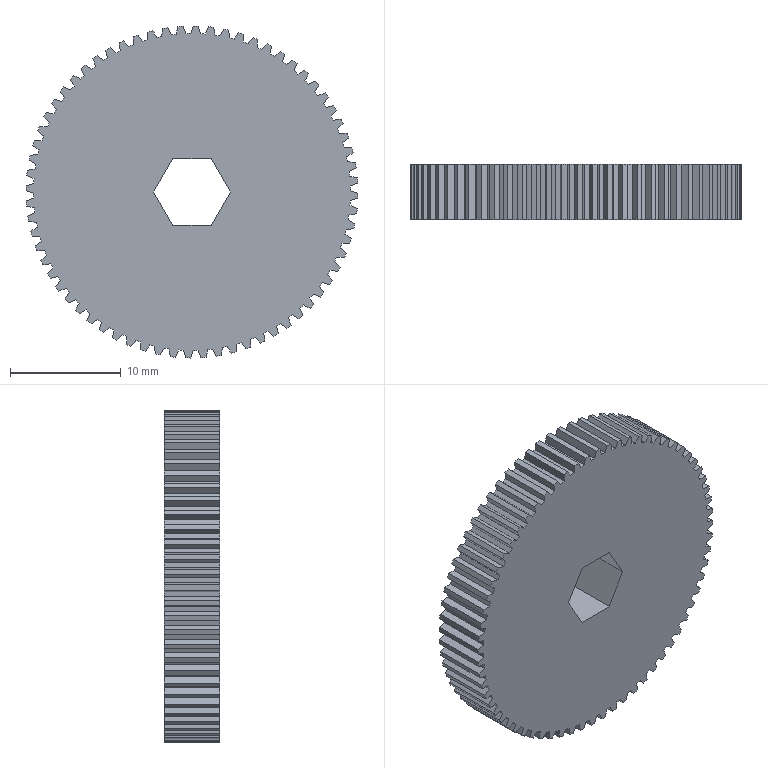Part | SolidWorks | features BaseBody 1 | 1 solid | 280 faces | box 29.999 x 5 x 29.999 mm | volume 3222 mm3 | plane 144 | cylinder 136 | commonest cylinder face diameters 28.654 x68 30 x68